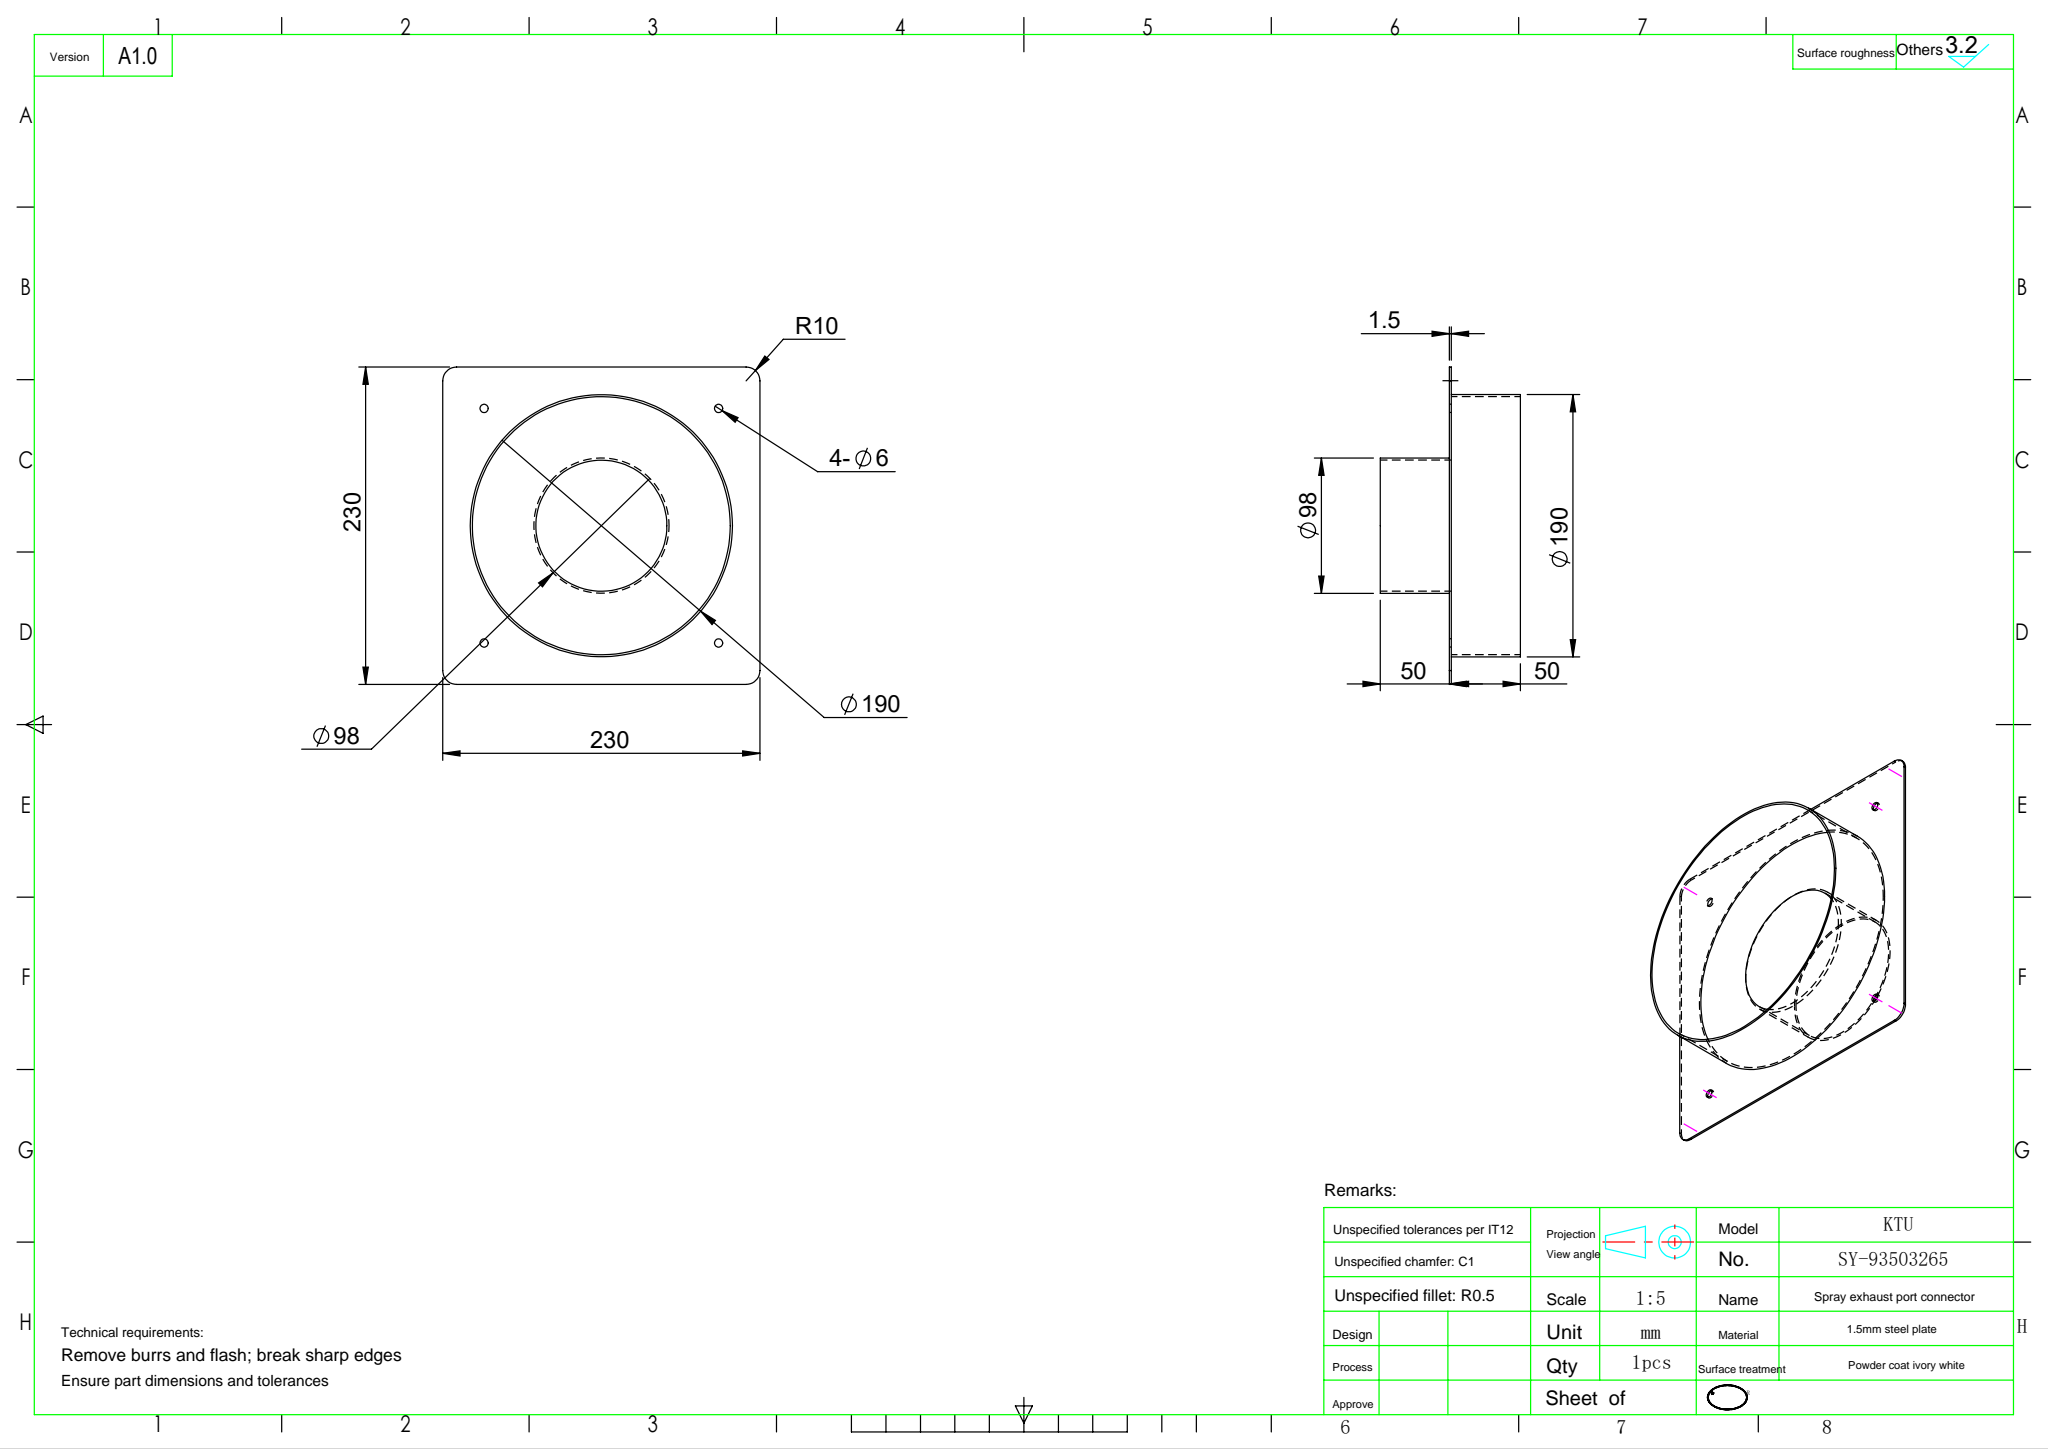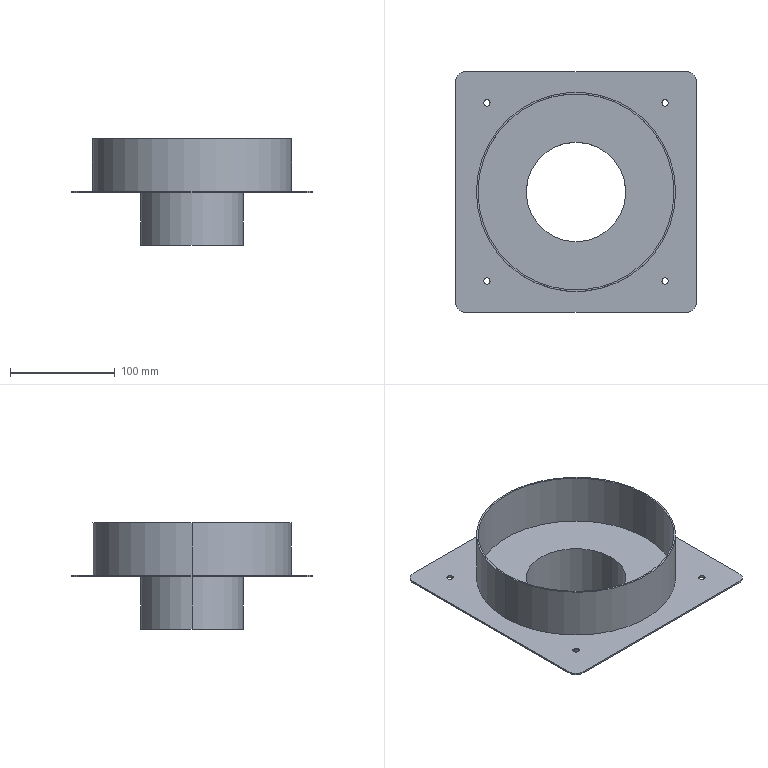Part | SolidWorks | features BossThin 2, FlatPattern 1, ICE 1, SMBaseFlange 1, SheetMetal 1 | 1 solid | 29 faces | box 230 x 230 x 101.5 mm | volume 135571 mm3 | cylinder 20 | plane 9 | commonest cylinder face diameters 6 x8 20 x4 95 x2 98 x2 187 x2 190 x2
STEP:
#1=CARTESIAN_POINT('',(-93.5,0.,50.));
#2=VERTEX_POINT('',#1);
#3=CARTESIAN_POINT('',(93.5,0.,50.));
#4=VERTEX_POINT('',#3);
#5=CARTESIAN_POINT('',(0.,0.,50.));
#6=DIRECTION('',(0.,0.,1.));
#7=DIRECTION('',(1.,0.,0.));
#8=AXIS2_PLACEMENT_3D('',#5,#6,#7);
#9=CIRCLE('',#8,93.5);
#10=EDGE_CURVE('',#2,#4,#9,.T.);
#11=ORIENTED_EDGE('',*,*,#10,.T.);
#12=CARTESIAN_POINT('',(93.5,0.,0.));
#13=VERTEX_POINT('',#12);
#14=CARTESIAN_POINT('',(93.5,0.,50.));
#15=DIRECTION('',(0.,0.,-1.));
#16=VECTOR('',#15,1000.);
#17=LINE('',#14,#16);
#18=EDGE_CURVE('',#4,#13,#17,.T.);
#19=ORIENTED_EDGE('',*,*,#18,.T.);
#20=CARTESIAN_POINT('',(-93.5,0.,0.));
#21=VERTEX_POINT('',#20);
#22=CARTESIAN_POINT('',(0.,0.,0.));
#23=DIRECTION('',(0.,0.,-1.));
#24=DIRECTION('',(1.,0.,0.));
#25=AXIS2_PLACEMENT_3D('',#22,#23,#24);
#26=CIRCLE('',#25,93.5);
#27=EDGE_CURVE('',#13,#21,#26,.T.);
#28=ORIENTED_EDGE('',*,*,#27,.T.);
#29=CARTESIAN_POINT('',(-93.5,0.,50.));
#30=DIRECTION('',(0.,0.,-1.));
#31=VECTOR('',#30,1000.);
#32=LINE('',#29,#31);
#33=EDGE_CURVE('',#2,#21,#32,.T.);
#34=ORIENTED_EDGE('',*,*,#33,.F.);
#35=EDGE_LOOP('',(#11,#19,#28,#34));
#36=FACE_OUTER_BOUND('',#35,.T.);
#37=CARTESIAN_POINT('',(0.,0.,50.));
#38=DIRECTION('',(0.,0.,-1.));
#39=DIRECTION('',(-1.,0.,0.));
#40=AXIS2_PLACEMENT_3D('',#37,#38,#39);
#41=CYLINDRICAL_SURFACE('',#40,93.5);
#42=ADVANCED_FACE('',(#36),#41,.F.);
#43=CARTESIAN_POINT('',(95.,0.,50.));
#44=VERTEX_POINT('',#43);
#45=CARTESIAN_POINT('',(-95.,0.,50.));
#46=VERTEX_POINT('',#45);
#47=CARTESIAN_POINT('',(0.,0.,50.));
#48=DIRECTION('',(0.,0.,1.));
#49=DIRECTION('',(1.,0.,0.));
#50=AXIS2_PLACEMENT_3D('',#47,#48,#49);
#51=CIRCLE('',#50,95.);
#52=EDGE_CURVE('',#44,#46,#51,.T.);
#53=ORIENTED_EDGE('',*,*,#52,.F.);
#54=CARTESIAN_POINT('',(95.,0.,0.));
#55=VERTEX_POINT('',#54);
#56=CARTESIAN_POINT('',(95.,0.,50.));
#57=DIRECTION('',(0.,0.,-1.));
#58=VECTOR('',#57,1000.);
#59=LINE('',#56,#58);
#60=EDGE_CURVE('',#44,#55,#59,.T.);
#61=ORIENTED_EDGE('',*,*,#60,.T.);
#62=CARTESIAN_POINT('',(-95.,0.,0.));
#63=VERTEX_POINT('',#62);
#64=CARTESIAN_POINT('',(0.,0.,0.));
#65=DIRECTION('',(0.,0.,1.));
#66=DIRECTION('',(1.,0.,0.));
#67=AXIS2_PLACEMENT_3D('',#64,#65,#66);
#68=CIRCLE('',#67,95.);
#69=EDGE_CURVE('',#55,#63,#68,.T.);
#70=ORIENTED_EDGE('',*,*,#69,.T.);
#71=CARTESIAN_POINT('',(-95.,0.,50.));
#72=DIRECTION('',(0.,0.,-1.));
#73=VECTOR('',#72,1000.);
#74=LINE('',#71,#73);
#75=EDGE_CURVE('',#46,#63,#74,.T.);
#76=ORIENTED_EDGE('',*,*,#75,.F.);
#77=EDGE_LOOP('',(#53,#61,#70,#76));
#78=FACE_OUTER_BOUND('',#77,.T.);
#79=CARTESIAN_POINT('',(0.,0.,50.));
#80=DIRECTION('',(0.,0.,-1.));
#81=DIRECTION('',(-1.,0.,0.));
#82=AXIS2_PLACEMENT_3D('',#79,#80,#81);
#83=CYLINDRICAL_SURFACE('',#82,95.);
#84=ADVANCED_FACE('',(#78),#83,.T.);
#85=CARTESIAN_POINT('',(-49.,0.,-51.5));
#86=VERTEX_POINT('',#85);
#87=CARTESIAN_POINT('',(49.,0.,-51.5));
#88=VERTEX_POINT('',#87);
#89=CARTESIAN_POINT('',(0.,0.,-51.5));
#90=DIRECTION('',(0.,0.,-1.));
#91=DIRECTION('',(-1.,0.,0.));
#92=AXIS2_PLACEMENT_3D('',#89,#90,#91);
#93=CIRCLE('',#92,49.);
#94=EDGE_CURVE('',#86,#88,#93,.T.);
#95=ORIENTED_EDGE('',*,*,#94,.F.);
#96=CARTESIAN_POINT('',(-49.,0.,-1.5));
#97=VERTEX_POINT('',#96);
#98=CARTESIAN_POINT('',(-49.,0.,-51.5));
#99=DIRECTION('',(0.,0.,1.));
#100=VECTOR('',#99,1000.);
#101=LINE('',#98,#100);
#102=EDGE_CURVE('',#86,#97,#101,.T.);
#103=ORIENTED_EDGE('',*,*,#102,.T.);
#104=CARTESIAN_POINT('',(49.,0.,-1.5));
#105=VERTEX_POINT('',#104);
#106=CARTESIAN_POINT('',(0.,0.,-1.5));
#107=DIRECTION('',(0.,0.,-1.));
#108=DIRECTION('',(1.,0.,0.));
#109=AXIS2_PLACEMENT_3D('',#106,#107,#108);
#110=CIRCLE('',#109,49.);
#111=EDGE_CURVE('',#97,#105,#110,.T.);
#112=ORIENTED_EDGE('',*,*,#111,.T.);
#113=CARTESIAN_POINT('',(49.,0.,-51.5));
#114=DIRECTION('',(0.,0.,1.));
#115=VECTOR('',#114,1000.);
#116=LINE('',#113,#115);
#117=EDGE_CURVE('',#88,#105,#116,.T.);
#118=ORIENTED_EDGE('',*,*,#117,.F.);
#119=EDGE_LOOP('',(#95,#103,#112,#118));
#120=FACE_OUTER_BOUND('',#119,.T.);
#121=CARTESIAN_POINT('',(0.,0.,-51.5));
#122=DIRECTION('',(0.,0.,1.));
#123=DIRECTION('',(1.,0.,0.));
#124=AXIS2_PLACEMENT_3D('',#121,#122,#123);
#125=CYLINDRICAL_SURFACE('',#124,49.);
#126=ADVANCED_FACE('',(#120),#125,.T.);
#127=CARTESIAN_POINT('',(82.,85.,0.));
#128=VERTEX_POINT('',#127);
#129=CARTESIAN_POINT('',(88.,85.,0.));
#130=VERTEX_POINT('',#129);
#131=CARTESIAN_POINT('',(85.,85.,0.));
#132=DIRECTION('',(0.,0.,1.));
#133=DIRECTION('',(1.,0.,0.));
#134=AXIS2_PLACEMENT_3D('',#131,#132,#133);
#135=CIRCLE('',#134,3.);
#136=EDGE_CURVE('',#128,#130,#135,.T.);
#137=ORIENTED_EDGE('',*,*,#136,.T.);
#138=CARTESIAN_POINT('',(88.,85.,-1.5));
#139=VERTEX_POINT('',#138);
#140=CARTESIAN_POINT('',(88.,85.,46.5));
#141=DIRECTION('',(0.,0.,-1.));
#142=VECTOR('',#141,1000.);
#143=LINE('',#140,#142);
#144=EDGE_CURVE('',#130,#139,#143,.T.);
#145=ORIENTED_EDGE('',*,*,#144,.T.);
#146=CARTESIAN_POINT('',(82.,85.,-1.5));
#147=VERTEX_POINT('',#146);
#148=CARTESIAN_POINT('',(85.,85.,-1.5));
#149=DIRECTION('',(0.,0.,-1.));
#150=DIRECTION('',(-1.,0.,0.));
#151=AXIS2_PLACEMENT_3D('',#148,#149,#150);
#152=CIRCLE('',#151,3.);
#153=EDGE_CURVE('',#139,#147,#152,.T.);
#154=ORIENTED_EDGE('',*,*,#153,.T.);
#155=CARTESIAN_POINT('',(82.,85.,46.5));
#156=DIRECTION('',(0.,0.,-1.));
#157=VECTOR('',#156,1000.);
#158=LINE('',#155,#157);
#159=EDGE_CURVE('',#128,#147,#158,.T.);
#160=ORIENTED_EDGE('',*,*,#159,.F.);
#161=EDGE_LOOP('',(#137,#145,#154,#160));
#162=FACE_OUTER_BOUND('',#161,.T.);
#163=CARTESIAN_POINT('',(85.,85.,46.5));
#164=DIRECTION('',(0.,0.,-1.));
#165=DIRECTION('',(-1.,0.,0.));
#166=AXIS2_PLACEMENT_3D('',#163,#164,#165);
#167=CYLINDRICAL_SURFACE('',#166,3.);
#168=ADVANCED_FACE('',(#162),#167,.F.);
#169=CARTESIAN_POINT('',(82.,-85.,0.));
#170=VERTEX_POINT('',#169);
#171=CARTESIAN_POINT('',(88.,-85.,0.));
#172=VERTEX_POINT('',#171);
#173=CARTESIAN_POINT('',(85.,-85.,0.));
#174=DIRECTION('',(0.,0.,1.));
#175=DIRECTION('',(1.,0.,0.));
#176=AXIS2_PLACEMENT_3D('',#173,#174,#175);
#177=CIRCLE('',#176,3.);
#178=EDGE_CURVE('',#170,#172,#177,.T.);
#179=ORIENTED_EDGE('',*,*,#178,.T.);
#180=CARTESIAN_POINT('',(88.,-85.,-1.5));
#181=VERTEX_POINT('',#180);
#182=CARTESIAN_POINT('',(88.,-85.,46.5));
#183=DIRECTION('',(0.,0.,-1.));
#184=VECTOR('',#183,1000.);
#185=LINE('',#182,#184);
#186=EDGE_CURVE('',#172,#181,#185,.T.);
#187=ORIENTED_EDGE('',*,*,#186,.T.);
#188=CARTESIAN_POINT('',(82.,-85.,-1.5));
#189=VERTEX_POINT('',#188);
#190=CARTESIAN_POINT('',(85.,-85.,-1.5));
#191=DIRECTION('',(0.,0.,-1.));
#192=DIRECTION('',(-1.,0.,0.));
#193=AXIS2_PLACEMENT_3D('',#190,#191,#192);
#194=CIRCLE('',#193,3.);
#195=EDGE_CURVE('',#181,#189,#194,.T.);
#196=ORIENTED_EDGE('',*,*,#195,.T.);
#197=CARTESIAN_POINT('',(82.,-85.,46.5));
#198=DIRECTION('',(0.,0.,-1.));
#199=VECTOR('',#198,1000.);
#200=LINE('',#197,#199);
#201=EDGE_CURVE('',#170,#189,#200,.T.);
#202=ORIENTED_EDGE('',*,*,#201,.F.);
#203=EDGE_LOOP('',(#179,#187,#196,#202));
#204=FACE_OUTER_BOUND('',#203,.T.);
#205=CARTESIAN_POINT('',(85.,-85.,46.5));
#206=DIRECTION('',(0.,0.,-1.));
#207=DIRECTION('',(-1.,0.,0.));
#208=AXIS2_PLACEMENT_3D('',#205,#206,#207);
#209=CYLINDRICAL_SURFACE('',#208,3.);
#210=ADVANCED_FACE('',(#204),#209,.F.);
#211=CARTESIAN_POINT('',(-88.,-85.,0.));
#212=VERTEX_POINT('',#211);
#213=CARTESIAN_POINT('',(-82.,-85.,0.));
#214=VERTEX_POINT('',#213);
#215=CARTESIAN_POINT('',(-85.,-85.,0.));
#216=DIRECTION('',(0.,0.,1.));
#217=DIRECTION('',(1.,0.,0.));
#218=AXIS2_PLACEMENT_3D('',#215,#216,#217);
#219=CIRCLE('',#218,3.);
#220=EDGE_CURVE('',#212,#214,#219,.T.);
#221=ORIENTED_EDGE('',*,*,#220,.T.);
#222=CARTESIAN_POINT('',(-82.,-85.,-1.5));
#223=VERTEX_POINT('',#222);
#224=CARTESIAN_POINT('',(-82.,-85.,46.5));
#225=DIRECTION('',(0.,0.,-1.));
#226=VECTOR('',#225,1000.);
#227=LINE('',#224,#226);
#228=EDGE_CURVE('',#214,#223,#227,.T.);
#229=ORIENTED_EDGE('',*,*,#228,.T.);
#230=CARTESIAN_POINT('',(-88.,-85.,-1.5));
#231=VERTEX_POINT('',#230);
#232=CARTESIAN_POINT('',(-85.,-85.,-1.5));
#233=DIRECTION('',(0.,0.,-1.));
#234=DIRECTION('',(-1.,0.,0.));
#235=AXIS2_PLACEMENT_3D('',#232,#233,#234);
#236=CIRCLE('',#235,3.);
#237=EDGE_CURVE('',#223,#231,#236,.T.);
#238=ORIENTED_EDGE('',*,*,#237,.T.);
#239=CARTESIAN_POINT('',(-88.,-85.,46.5));
#240=DIRECTION('',(0.,0.,-1.));
#241=VECTOR('',#240,1000.);
#242=LINE('',#239,#241);
#243=EDGE_CURVE('',#212,#231,#242,.T.);
#244=ORIENTED_EDGE('',*,*,#243,.F.);
#245=EDGE_LOOP('',(#221,#229,#238,#244));
#246=FACE_OUTER_BOUND('',#245,.T.);
#247=CARTESIAN_POINT('',(-85.,-85.,46.5));
#248=DIRECTION('',(0.,0.,-1.));
#249=DIRECTION('',(-1.,0.,0.));
#250=AXIS2_PLACEMENT_3D('',#247,#248,#249);
#251=CYLINDRICAL_SURFACE('',#250,3.);
#252=ADVANCED_FACE('',(#246),#251,.F.);
#253=CARTESIAN_POINT('',(-88.,85.,0.));
#254=VERTEX_POINT('',#253);
#255=CARTESIAN_POINT('',(-82.,85.,0.));
#256=VERTEX_POINT('',#255);
#257=CARTESIAN_POINT('',(-85.,85.,0.));
#258=DIRECTION('',(0.,0.,1.));
#259=DIRECTION('',(1.,0.,0.));
#260=AXIS2_PLACEMENT_3D('',#257,#258,#259);
#261=CIRCLE('',#260,3.);
#262=EDGE_CURVE('',#254,#256,#261,.T.);
#263=ORIENTED_EDGE('',*,*,#262,.T.);
#264=CARTESIAN_POINT('',(-82.,85.,-1.5));
#265=VERTEX_POINT('',#264);
#266=CARTESIAN_POINT('',(-82.,85.,46.5));
#267=DIRECTION('',(0.,0.,-1.));
#268=VECTOR('',#267,1000.);
#269=LINE('',#266,#268);
#270=EDGE_CURVE('',#256,#265,#269,.T.);
#271=ORIENTED_EDGE('',*,*,#270,.T.);
#272=CARTESIAN_POINT('',(-88.,85.,-1.5));
#273=VERTEX_POINT('',#272);
#274=CARTESIAN_POINT('',(-85.,85.,-1.5));
#275=DIRECTION('',(0.,0.,-1.));
#276=DIRECTION('',(-1.,0.,0.));
#277=AXIS2_PLACEMENT_3D('',#274,#275,#276);
#278=CIRCLE('',#277,3.);
#279=EDGE_CURVE('',#265,#273,#278,.T.);
#280=ORIENTED_EDGE('',*,*,#279,.T.);
#281=CARTESIAN_POINT('',(-88.,85.,46.5));
#282=DIRECTION('',(0.,0.,-1.));
#283=VECTOR('',#282,1000.);
#284=LINE('',#281,#283);
#285=EDGE_CURVE('',#254,#273,#284,.T.);
#286=ORIENTED_EDGE('',*,*,#285,.F.);
#287=EDGE_LOOP('',(#263,#271,#280,#286));
#288=FACE_OUTER_BOUND('',#287,.T.);
#289=CARTESIAN_POINT('',(-85.,85.,46.5));
#290=DIRECTION('',(0.,0.,-1.));
#291=DIRECTION('',(-1.,0.,0.));
#292=AXIS2_PLACEMENT_3D('',#289,#290,#291);
#293=CYLINDRICAL_SURFACE('',#292,3.);
#294=ADVANCED_FACE('',(#288),#293,.F.);
#295=CARTESIAN_POINT('',(47.5,0.,-51.5));
#296=VERTEX_POINT('',#295);
#297=CARTESIAN_POINT('',(-47.5,0.,-51.5));
#298=VERTEX_POINT('',#297);
#299=CARTESIAN_POINT('',(0.,0.,-51.5));
#300=DIRECTION('',(0.,0.,-1.));
#301=DIRECTION('',(-1.,0.,0.));
#302=AXIS2_PLACEMENT_3D('',#299,#300,#301);
#303=CIRCLE('',#302,47.5);
#304=EDGE_CURVE('',#296,#298,#303,.T.);
#305=ORIENTED_EDGE('',*,*,#304,.T.);
#306=CARTESIAN_POINT('',(-47.5,0.,0.));
#307=VERTEX_POINT('',#306);
#308=CARTESIAN_POINT('',(-47.5,0.,-1.5));
#309=DIRECTION('',(0.,0.,1.));
#310=VECTOR('',#309,1000.);
#311=LINE('',#308,#310);
#312=EDGE_CURVE('',#298,#307,#311,.T.);
#313=ORIENTED_EDGE('',*,*,#312,.T.);
#314=CARTESIAN_POINT('',(47.5,0.,0.));
#315=VERTEX_POINT('',#314);
#316=CARTESIAN_POINT('',(0.,0.,0.));
#317=DIRECTION('',(0.,0.,1.));
#318=DIRECTION('',(1.,0.,0.));
#319=AXIS2_PLACEMENT_3D('',#316,#317,#318);
#320=CIRCLE('',#319,47.5);
#321=EDGE_CURVE('',#307,#315,#320,.T.);
#322=ORIENTED_EDGE('',*,*,#321,.T.);
#323=CARTESIAN_POINT('',(47.5,0.,-1.5));
#324=DIRECTION('',(0.,0.,1.));
#325=VECTOR('',#324,1000.);
#326=LINE('',#323,#325);
#327=EDGE_CURVE('',#296,#315,#326,.T.);
#328=ORIENTED_EDGE('',*,*,#327,.F.);
#329=EDGE_LOOP('',(#305,#313,#322,#328));
#330=FACE_OUTER_BOUND('',#329,.T.);
#331=CARTESIAN_POINT('',(0.,0.,-1.5));
#332=DIRECTION('',(0.,0.,1.));
#333=DIRECTION('',(1.,0.,0.));
#334=AXIS2_PLACEMENT_3D('',#331,#332,#333);
#335=CYLINDRICAL_SURFACE('',#334,47.5);
#336=ADVANCED_FACE('',(#330),#335,.F.);
#337=CARTESIAN_POINT('',(0.,0.,0.));
#338=DIRECTION('',(0.,0.,1.));
#339=DIRECTION('',(1.,0.,0.));
#340=AXIS2_PLACEMENT_3D('',#337,#338,#339);
#341=CIRCLE('',#340,47.5);
#342=EDGE_CURVE('',#315,#307,#341,.T.);
#343=ORIENTED_EDGE('',*,*,#342,.F.);
#344=ORIENTED_EDGE('',*,*,#321,.F.);
#345=EDGE_LOOP('',(#343,#344));
#346=FACE_BOUND('',#345,.T.);
#347=CARTESIAN_POINT('',(0.,0.,0.));
#348=DIRECTION('',(0.,0.,-1.));
#349=DIRECTION('',(1.,0.,0.));
#350=AXIS2_PLACEMENT_3D('',#347,#348,#349);
#351=CIRCLE('',#350,93.5);
#352=EDGE_CURVE('',#21,#13,#351,.T.);
#353=ORIENTED_EDGE('',*,*,#352,.F.);
#354=ORIENTED_EDGE('',*,*,#27,.F.);
#355=EDGE_LOOP('',(#353,#354));
#356=FACE_OUTER_BOUND('',#355,.T.);
#357=CARTESIAN_POINT('',(-105.,-105.,0.));
#358=DIRECTION('',(0.,0.,1.));
#359=DIRECTION('',(1.,0.,0.));
#360=AXIS2_PLACEMENT_3D('',#357,#358,#359);
#361=PLANE('',#360);
#362=ADVANCED_FACE('',(#346,#356),#361,.T.);
#363=CARTESIAN_POINT('',(-115.,-105.,-1.5));
#364=VERTEX_POINT('',#363);
#365=CARTESIAN_POINT('',(-105.,-115.,-1.5));
#366=VERTEX_POINT('',#365);
#367=CARTESIAN_POINT('',(-105.,-105.,-1.5));
#368=DIRECTION('',(0.,0.,1.));
#369=DIRECTION('',(1.,0.,0.));
#370=AXIS2_PLACEMENT_3D('',#367,#368,#369);
#371=CIRCLE('',#370,10.);
#372=EDGE_CURVE('',#364,#366,#371,.T.);
#373=ORIENTED_EDGE('',*,*,#372,.F.);
#374=CARTESIAN_POINT('',(-115.,105.,-1.5));
#375=VERTEX_POINT('',#374);
#376=CARTESIAN_POINT('',(-115.,-105.,-1.5));
#377=DIRECTION('',(0.,-1.,0.));
#378=VECTOR('',#377,1000.);
#379=LINE('',#376,#378);
#380=EDGE_CURVE('',#375,#364,#379,.T.);
#381=ORIENTED_EDGE('',*,*,#380,.F.);
#382=CARTESIAN_POINT('',(-105.,115.,-1.5));
#383=VERTEX_POINT('',#382);
#384=CARTESIAN_POINT('',(-105.,105.,-1.5));
#385=DIRECTION('',(0.,0.,1.));
#386=DIRECTION('',(-1.,0.,0.));
#387=AXIS2_PLACEMENT_3D('',#384,#385,#386);
#388=CIRCLE('',#387,10.);
#389=EDGE_CURVE('',#383,#375,#388,.T.);
#390=ORIENTED_EDGE('',*,*,#389,.F.);
#391=CARTESIAN_POINT('',(105.,115.,-1.5));
#392=VERTEX_POINT('',#391);
#393=CARTESIAN_POINT('',(-105.,115.,-1.5));
#394=DIRECTION('',(-1.,0.,0.));
#395=VECTOR('',#394,1000.);
#396=LINE('',#393,#395);
#397=EDGE_CURVE('',#392,#383,#396,.T.);
#398=ORIENTED_EDGE('',*,*,#397,.F.);
#399=CARTESIAN_POINT('',(115.,105.,-1.5));
#400=VERTEX_POINT('',#399);
#401=CARTESIAN_POINT('',(105.,105.,-1.5));
#402=DIRECTION('',(0.,0.,1.));
#403=DIRECTION('',(1.,0.,0.));
#404=AXIS2_PLACEMENT_3D('',#401,#402,#403);
#405=CIRCLE('',#404,10.);
#406=EDGE_CURVE('',#400,#392,#405,.T.);
#407=ORIENTED_EDGE('',*,*,#406,.F.);
#408=CARTESIAN_POINT('',(115.,-105.,-1.5));
#409=VERTEX_POINT('',#408);
#410=CARTESIAN_POINT('',(115.,-105.,-1.5));
#411=DIRECTION('',(0.,1.,0.));
#412=VECTOR('',#411,1000.);
#413=LINE('',#410,#412);
#414=EDGE_CURVE('',#409,#400,#413,.T.);
#415=ORIENTED_EDGE('',*,*,#414,.F.);
#416=CARTESIAN_POINT('',(105.,-115.,-1.5));
#417=VERTEX_POINT('',#416);
#418=CARTESIAN_POINT('',(105.,-105.,-1.5));
#419=DIRECTION('',(0.,0.,1.));
#420=DIRECTION('',(1.,0.,0.));
#421=AXIS2_PLACEMENT_3D('',#418,#419,#420);
#422=CIRCLE('',#421,10.);
#423=EDGE_CURVE('',#417,#409,#422,.T.);
#424=ORIENTED_EDGE('',*,*,#423,.F.);
#425=CARTESIAN_POINT('',(-105.,-115.,-1.5));
#426=DIRECTION('',(1.,0.,0.));
#427=VECTOR('',#426,1000.);
#428=LINE('',#425,#427);
#429=EDGE_CURVE('',#366,#417,#428,.T.);
#430=ORIENTED_EDGE('',*,*,#429,.F.);
#431=EDGE_LOOP('',(#373,#381,#390,#398,#407,#415,#424,#430));
#432=FACE_OUTER_BOUND('',#431,.T.);
#433=CARTESIAN_POINT('',(-85.,85.,-1.5));
#434=DIRECTION('',(0.,0.,-1.));
#435=DIRECTION('',(-1.,0.,0.));
#436=AXIS2_PLACEMENT_3D('',#433,#434,#435);
#437=CIRCLE('',#436,3.);
#438=EDGE_CURVE('',#273,#265,#437,.T.);
#439=ORIENTED_EDGE('',*,*,#438,.F.);
#440=ORIENTED_EDGE('',*,*,#279,.F.);
#441=EDGE_LOOP('',(#439,#440));
#442=FACE_BOUND('',#441,.T.);
#443=CARTESIAN_POINT('',(-85.,-85.,-1.5));
#444=DIRECTION('',(0.,0.,-1.));
#445=DIRECTION('',(-1.,0.,0.));
#446=AXIS2_PLACEMENT_3D('',#443,#444,#445);
#447=CIRCLE('',#446,3.);
#448=EDGE_CURVE('',#231,#223,#447,.T.);
#449=ORIENTED_EDGE('',*,*,#448,.F.);
#450=ORIENTED_EDGE('',*,*,#237,.F.);
#451=EDGE_LOOP('',(#449,#450));
#452=FACE_BOUND('',#451,.T.);
#453=CARTESIAN_POINT('',(85.,-85.,-1.5));
#454=DIRECTION('',(0.,0.,-1.));
#455=DIRECTION('',(-1.,0.,0.));
#456=AXIS2_PLACEMENT_3D('',#453,#454,#455);
#457=CIRCLE('',#456,3.);
#458=EDGE_CURVE('',#189,#181,#457,.T.);
#459=ORIENTED_EDGE('',*,*,#458,.F.);
#460=ORIENTED_EDGE('',*,*,#195,.F.);
#461=EDGE_LOOP('',(#459,#460));
#462=FACE_BOUND('',#461,.T.);
#463=CARTESIAN_POINT('',(85.,85.,-1.5));
#464=DIRECTION('',(0.,0.,-1.));
#465=DIRECTION('',(-1.,0.,0.));
#466=AXIS2_PLACEMENT_3D('',#463,#464,#465);
#467=CIRCLE('',#466,3.);
#468=EDGE_CURVE('',#147,#139,#467,.T.);
#469=ORIENTED_EDGE('',*,*,#468,.F.);
#470=ORIENTED_EDGE('',*,*,#153,.F.);
#471=EDGE_LOOP('',(#469,#470));
#472=FACE_BOUND('',#471,.T.);
#473=CARTESIAN_POINT('',(0.,0.,-1.5));
#474=DIRECTION('',(0.,0.,-1.));
#475=DIRECTION('',(1.,0.,0.));
#476=AXIS2_PLACEMENT_3D('',#473,#474,#475);
#477=CIRCLE('',#476,49.);
#478=EDGE_CURVE('',#105,#97,#477,.T.);
#479=ORIENTED_EDGE('',*,*,#478,.F.);
#480=ORIENTED_EDGE('',*,*,#111,.F.);
#481=EDGE_LOOP('',(#479,#480));
#482=FACE_BOUND('',#481,.T.);
#483=CARTESIAN_POINT('',(-105.,-105.,-1.5));
#484=DIRECTION('',(0.,0.,1.));
#485=DIRECTION('',(1.,0.,0.));
#486=AXIS2_PLACEMENT_3D('',#483,#484,#485);
#487=PLANE('',#486);
#488=ADVANCED_FACE('',(#432,#442,#452,#462,#472,#482),#487,.F.);
#489=CARTESIAN_POINT('',(-115.,-105.,0.));
#490=VERTEX_POINT('',#489);
#491=CARTESIAN_POINT('',(-105.,-115.,0.));
#492=VERTEX_POINT('',#491);
#493=CARTESIAN_POINT('',(-105.,-105.,0.));
#494=DIRECTION('',(0.,0.,1.));
#495=DIRECTION('',(1.,0.,0.));
#496=AXIS2_PLACEMENT_3D('',#493,#494,#495);
#497=CIRCLE('',#496,10.);
#498=EDGE_CURVE('',#490,#492,#497,.T.);
#499=ORIENTED_EDGE('',*,*,#498,.F.);
#500=CARTESIAN_POINT('',(-115.,-105.,-1.5));
#501=DIRECTION('',(0.,0.,1.));
#502=VECTOR('',#501,1000.);
#503=LINE('',#500,#502);
#504=EDGE_CURVE('',#364,#490,#503,.T.);
#505=ORIENTED_EDGE('',*,*,#504,.F.);
#506=ORIENTED_EDGE('',*,*,#372,.T.);
#507=CARTESIAN_POINT('',(-105.,-115.,-1.5));
#508=DIRECTION('',(0.,0.,1.));
#509=VECTOR('',#508,1000.);
#510=LINE('',#507,#509);
#511=EDGE_CURVE('',#366,#492,#510,.T.);
#512=ORIENTED_EDGE('',*,*,#511,.T.);
#513=EDGE_LOOP('',(#499,#505,#506,#512));
#514=FACE_OUTER_BOUND('',#513,.T.);
#515=CARTESIAN_POINT('',(-105.,-105.,-1.5));
#516=DIRECTION('',(0.,0.,1.));
#517=DIRECTION('',(1.,0.,0.));
#518=AXIS2_PLACEMENT_3D('',#515,#516,#517);
#519=CYLINDRICAL_SURFACE('',#518,10.);
#520=ADVANCED_FACE('',(#514),#519,.T.);
#521=CARTESIAN_POINT('',(-115.,105.,0.));
#522=VERTEX_POINT('',#521);
#523=CARTESIAN_POINT('',(-115.,-105.,0.));
#524=DIRECTION('',(0.,-1.,0.));
#525=VECTOR('',#524,1000.);
#526=LINE('',#523,#525);
#527=EDGE_CURVE('',#522,#490,#526,.T.);
#528=ORIENTED_EDGE('',*,*,#527,.F.);
#529=CARTESIAN_POINT('',(-115.,105.,-1.5));
#530=DIRECTION('',(0.,0.,1.));
#531=VECTOR('',#530,1000.);
#532=LINE('',#529,#531);
#533=EDGE_CURVE('',#375,#522,#532,.T.);
#534=ORIENTED_EDGE('',*,*,#533,.F.);
#535=ORIENTED_EDGE('',*,*,#380,.T.);
#536=ORIENTED_EDGE('',*,*,#504,.T.);
#537=EDGE_LOOP('',(#528,#534,#535,#536));
#538=FACE_OUTER_BOUND('',#537,.T.);
#539=CARTESIAN_POINT('',(-115.,-105.,-1.5));
#540=DIRECTION('',(-1.,0.,0.));
#541=DIRECTION('',(0.,0.,1.));
#542=AXIS2_PLACEMENT_3D('',#539,#540,#541);
#543=PLANE('',#542);
#544=ADVANCED_FACE('',(#538),#543,.T.);
#545=CARTESIAN_POINT('',(-105.,115.,0.));
#546=VERTEX_POINT('',#545);
#547=CARTESIAN_POINT('',(-105.,105.,0.));
#548=DIRECTION('',(0.,0.,1.));
#549=DIRECTION('',(-1.,0.,0.));
#550=AXIS2_PLACEMENT_3D('',#547,#548,#549);
#551=CIRCLE('',#550,10.);
#552=EDGE_CURVE('',#546,#522,#551,.T.);
#553=ORIENTED_EDGE('',*,*,#552,.F.);
#554=CARTESIAN_POINT('',(-105.,115.,-1.5));
#555=DIRECTION('',(0.,0.,1.));
#556=VECTOR('',#555,1000.);
#557=LINE('',#554,#556);
#558=EDGE_CURVE('',#383,#546,#557,.T.);
#559=ORIENTED_EDGE('',*,*,#558,.F.);
#560=ORIENTED_EDGE('',*,*,#389,.T.);
#561=ORIENTED_EDGE('',*,*,#533,.T.);
#562=EDGE_LOOP('',(#553,#559,#560,#561));
#563=FACE_OUTER_BOUND('',#562,.T.);
#564=CARTESIAN_POINT('',(-105.,105.,-1.5));
#565=DIRECTION('',(0.,0.,1.));
#566=DIRECTION('',(1.,0.,0.));
#567=AXIS2_PLACEMENT_3D('',#564,#565,#566);
#568=CYLINDRICAL_SURFACE('',#567,10.);
#569=ADVANCED_FACE('',(#563),#568,.T.);
#570=CARTESIAN_POINT('',(105.,115.,0.));
#571=VERTEX_POINT('',#570);
#572=CARTESIAN_POINT('',(-105.,115.,0.));
#573=DIRECTION('',(-1.,0.,0.));
#574=VECTOR('',#573,1000.);
#575=LINE('',#572,#574);
#576=EDGE_CURVE('',#571,#546,#575,.T.);
#577=ORIENTED_EDGE('',*,*,#576,.F.);
#578=CARTESIAN_POINT('',(105.,115.,-1.5));
#579=DIRECTION('',(0.,0.,1.));
#580=VECTOR('',#579,1000.);
#581=LINE('',#578,#580);
#582=EDGE_CURVE('',#392,#571,#581,.T.);
#583=ORIENTED_EDGE('',*,*,#582,.F.);
#584=ORIENTED_EDGE('',*,*,#397,.T.);
#585=ORIENTED_EDGE('',*,*,#558,.T.);
#586=EDGE_LOOP('',(#577,#583,#584,#585));
#587=FACE_OUTER_BOUND('',#586,.T.);
#588=CARTESIAN_POINT('',(-105.,115.,-1.5));
#589=DIRECTION('',(0.,1.,0.));
#590=DIRECTION('',(0.,0.,1.));
#591=AXIS2_PLACEMENT_3D('',#588,#589,#590);
#592=PLANE('',#591);
#593=ADVANCED_FACE('',(#587),#592,.T.);
#594=CARTESIAN_POINT('',(115.,105.,0.));
#595=VERTEX_POINT('',#594);
#596=CARTESIAN_POINT('',(105.,105.,0.));
#597=DIRECTION('',(0.,0.,1.));
#598=DIRECTION('',(1.,0.,0.));
#599=AXIS2_PLACEMENT_3D('',#596,#597,#598);
#600=CIRCLE('',#599,10.);
#601=EDGE_CURVE('',#595,#571,#600,.T.);
#602=ORIENTED_EDGE('',*,*,#601,.F.);
#603=CARTESIAN_POINT('',(115.,105.,-1.5));
#604=DIRECTION('',(0.,0.,1.));
#605=VECTOR('',#604,1000.);
#606=LINE('',#603,#605);
#607=EDGE_CURVE('',#400,#595,#606,.T.);
#608=ORIENTED_EDGE('',*,*,#607,.F.);
#609=ORIENTED_EDGE('',*,*,#406,.T.);
#610=ORIENTED_EDGE('',*,*,#582,.T.);
#611=EDGE_LOOP('',(#602,#608,#609,#610));
#612=FACE_OUTER_BOUND('',#611,.T.);
#613=CARTESIAN_POINT('',(105.,105.,-1.5));
#614=DIRECTION('',(0.,0.,1.));
#615=DIRECTION('',(1.,0.,0.));
#616=AXIS2_PLACEMENT_3D('',#613,#614,#615);
#617=CYLINDRICAL_SURFACE('',#616,10.);
#618=ADVANCED_FACE('',(#612),#617,.T.);
#619=CARTESIAN_POINT('',(115.,-105.,0.));
#620=VERTEX_POINT('',#619);
#621=CARTESIAN_POINT('',(115.,-105.,0.));
#622=DIRECTION('',(0.,1.,0.));
#623=VECTOR('',#622,1000.);
#624=LINE('',#621,#623);
#625=EDGE_CURVE('',#620,#595,#624,.T.);
#626=ORIENTED_EDGE('',*,*,#625,.F.);
#627=CARTESIAN_POINT('',(115.,-105.,-1.5));
#628=DIRECTION('',(0.,0.,1.));
#629=VECTOR('',#628,1000.);
#630=LINE('',#627,#629);
#631=EDGE_CURVE('',#409,#620,#630,.T.);
#632=ORIENTED_EDGE('',*,*,#631,.F.);
#633=ORIENTED_EDGE('',*,*,#414,.T.);
#634=ORIENTED_EDGE('',*,*,#607,.T.);
#635=EDGE_LOOP('',(#626,#632,#633,#634));
#636=FACE_OUTER_BOUND('',#635,.T.);
#637=CARTESIAN_POINT('',(115.,-105.,-1.5));
#638=DIRECTION('',(1.,0.,0.));
#639=DIRECTION('',(0.,0.,-1.));
#640=AXIS2_PLACEMENT_3D('',#637,#638,#639);
#641=PLANE('',#640);
#642=ADVANCED_FACE('',(#636),#641,.T.);
#643=CARTESIAN_POINT('',(105.,-115.,0.));
#644=VERTEX_POINT('',#643);
#645=CARTESIAN_POINT('',(105.,-105.,0.));
#646=DIRECTION('',(0.,0.,1.));
#647=DIRECTION('',(1.,0.,0.));
#648=AXIS2_PLACEMENT_3D('',#645,#646,#647);
#649=CIRCLE('',#648,10.);
#650=EDGE_CURVE('',#644,#620,#649,.T.);
#651=ORIENTED_EDGE('',*,*,#650,.F.);
#652=CARTESIAN_POINT('',(105.,-115.,-1.5));
#653=DIRECTION('',(0.,0.,1.));
#654=VECTOR('',#653,1000.);
#655=LINE('',#652,#654);
#656=EDGE_CURVE('',#417,#644,#655,.T.);
#657=ORIENTED_EDGE('',*,*,#656,.F.);
#658=ORIENTED_EDGE('',*,*,#423,.T.);
#659=ORIENTED_EDGE('',*,*,#631,.T.);
#660=EDGE_LOOP('',(#651,#657,#658,#659));
#661=FACE_OUTER_BOUND('',#660,.T.);
#662=CARTESIAN_POINT('',(105.,-105.,-1.5));
#663=DIRECTION('',(0.,0.,1.));
#664=DIRECTION('',(1.,0.,0.));
#665=AXIS2_PLACEMENT_3D('',#662,#663,#664);
#666=CYLINDRICAL_SURFACE('',#665,10.);
#667=ADVANCED_FACE('',(#661),#666,.T.);
#668=CARTESIAN_POINT('',(-105.,-115.,0.));
#669=DIRECTION('',(1.,0.,0.));
#670=VECTOR('',#669,1000.);
#671=LINE('',#668,#670);
#672=EDGE_CURVE('',#492,#644,#671,.T.);
#673=ORIENTED_EDGE('',*,*,#672,.F.);
#674=ORIENTED_EDGE('',*,*,#511,.F.);
#675=ORIENTED_EDGE('',*,*,#429,.T.);
#676=ORIENTED_EDGE('',*,*,#656,.T.);
#677=EDGE_LOOP('',(#673,#674,#675,#676));
#678=FACE_OUTER_BOUND('',#677,.T.);
#679=CARTESIAN_POINT('',(-105.,-115.,-1.5));
#680=DIRECTION('',(0.,-1.,0.));
#681=DIRECTION('',(0.,0.,-1.));
#682=AXIS2_PLACEMENT_3D('',#679,#680,#681);
#683=PLANE('',#682);
#684=ADVANCED_FACE('',(#678),#683,.T.);
#685=CARTESIAN_POINT('',(0.,0.,0.));
#686=DIRECTION('',(0.,0.,1.));
#687=DIRECTION('',(1.,0.,0.));
#688=AXIS2_PLACEMENT_3D('',#685,#686,#687);
#689=CIRCLE('',#688,95.);
#690=EDGE_CURVE('',#63,#55,#689,.T.);
#691=ORIENTED_EDGE('',*,*,#690,.F.);
#692=ORIENTED_EDGE('',*,*,#69,.F.);
#693=EDGE_LOOP('',(#691,#692));
#694=FACE_BOUND('',#693,.T.);
#695=ORIENTED_EDGE('',*,*,#136,.F.);
#696=CARTESIAN_POINT('',(85.,85.,0.));
#697=DIRECTION('',(0.,0.,1.));
#698=DIRECTION('',(1.,0.,0.));
#699=AXIS2_PLACEMENT_3D('',#696,#697,#698);
#700=CIRCLE('',#699,3.);
#701=EDGE_CURVE('',#130,#128,#700,.T.);
#702=ORIENTED_EDGE('',*,*,#701,.F.);
#703=EDGE_LOOP('',(#695,#702));
#704=FACE_BOUND('',#703,.T.);
#705=ORIENTED_EDGE('',*,*,#178,.F.);
#706=CARTESIAN_POINT('',(85.,-85.,0.));
#707=DIRECTION('',(0.,0.,1.));
#708=DIRECTION('',(1.,0.,0.));
#709=AXIS2_PLACEMENT_3D('',#706,#707,#708);
#710=CIRCLE('',#709,3.);
#711=EDGE_CURVE('',#172,#170,#710,.T.);
#712=ORIENTED_EDGE('',*,*,#711,.F.);
#713=EDGE_LOOP('',(#705,#712));
#714=FACE_BOUND('',#713,.T.);
#715=ORIENTED_EDGE('',*,*,#220,.F.);
#716=CARTESIAN_POINT('',(-85.,-85.,0.));
#717=DIRECTION('',(0.,0.,1.));
#718=DIRECTION('',(1.,0.,0.));
#719=AXIS2_PLACEMENT_3D('',#716,#717,#718);
#720=CIRCLE('',#719,3.);
#721=EDGE_CURVE('',#214,#212,#720,.T.);
#722=ORIENTED_EDGE('',*,*,#721,.F.);
#723=EDGE_LOOP('',(#715,#722));
#724=FACE_BOUND('',#723,.T.);
#725=ORIENTED_EDGE('',*,*,#262,.F.);
#726=CARTESIAN_POINT('',(-85.,85.,0.));
#727=DIRECTION('',(0.,0.,1.));
#728=DIRECTION('',(1.,0.,0.));
#729=AXIS2_PLACEMENT_3D('',#726,#727,#728);
#730=CIRCLE('',#729,3.);
#731=EDGE_CURVE('',#256,#254,#730,.T.);
#732=ORIENTED_EDGE('',*,*,#731,.F.);
#733=EDGE_LOOP('',(#725,#732));
#734=FACE_BOUND('',#733,.T.);
#735=ORIENTED_EDGE('',*,*,#498,.T.);
#736=ORIENTED_EDGE('',*,*,#672,.T.);
#737=ORIENTED_EDGE('',*,*,#650,.T.);
#738=ORIENTED_EDGE('',*,*,#625,.T.);
#739=ORIENTED_EDGE('',*,*,#601,.T.);
#740=ORIENTED_EDGE('',*,*,#576,.T.);
#741=ORIENTED_EDGE('',*,*,#552,.T.);
#742=ORIENTED_EDGE('',*,*,#527,.T.);
#743=EDGE_LOOP('',(#735,#736,#737,#738,#739,#740,#741,#742));
#744=FACE_OUTER_BOUND('',#743,.T.);
#745=CARTESIAN_POINT('',(-105.,-105.,0.));
#746=DIRECTION('',(0.,0.,1.));
#747=DIRECTION('',(1.,0.,0.));
#748=AXIS2_PLACEMENT_3D('',#745,#746,#747);
#749=PLANE('',#748);
#750=ADVANCED_FACE('',(#694,#704,#714,#724,#734,#744),#749,.T.);
#751=ORIENTED_EDGE('',*,*,#312,.F.);
#752=CARTESIAN_POINT('',(0.,0.,-51.5));
#753=DIRECTION('',(0.,0.,-1.));
#754=DIRECTION('',(-1.,0.,0.));
#755=AXIS2_PLACEMENT_3D('',#752,#753,#754);
#756=CIRCLE('',#755,47.5);
#757=EDGE_CURVE('',#298,#296,#756,.T.);
#758=ORIENTED_EDGE('',*,*,#757,.T.);
#759=ORIENTED_EDGE('',*,*,#327,.T.);
#760=ORIENTED_EDGE('',*,*,#342,.T.);
#761=EDGE_LOOP('',(#751,#758,#759,#760));
#762=FACE_OUTER_BOUND('',#761,.T.);
#763=CARTESIAN_POINT('',(0.,0.,-1.5));
#764=DIRECTION('',(0.,0.,1.));
#765=DIRECTION('',(1.,0.,0.));
#766=AXIS2_PLACEMENT_3D('',#763,#764,#765);
#767=CYLINDRICAL_SURFACE('',#766,47.5);
#768=ADVANCED_FACE('',(#762),#767,.F.);
#769=ORIENTED_EDGE('',*,*,#270,.F.);
#770=ORIENTED_EDGE('',*,*,#731,.T.);
#771=ORIENTED_EDGE('',*,*,#285,.T.);
#772=ORIENTED_EDGE('',*,*,#438,.T.);
#773=EDGE_LOOP('',(#769,#770,#771,#772));
#774=FACE_OUTER_BOUND('',#773,.T.);
#775=CARTESIAN_POINT('',(-85.,85.,46.5));
#776=DIRECTION('',(0.,0.,-1.));
#777=DIRECTION('',(-1.,0.,0.));
#778=AXIS2_PLACEMENT_3D('',#775,#776,#777);
#779=CYLINDRICAL_SURFACE('',#778,3.);
#780=ADVANCED_FACE('',(#774),#779,.F.);
#781=ORIENTED_EDGE('',*,*,#228,.F.);
#782=ORIENTED_EDGE('',*,*,#721,.T.);
#783=ORIENTED_EDGE('',*,*,#243,.T.);
#784=ORIENTED_EDGE('',*,*,#448,.T.);
#785=EDGE_LOOP('',(#781,#782,#783,#784));
#786=FACE_OUTER_BOUND('',#785,.T.);
#787=CARTESIAN_POINT('',(-85.,-85.,46.5));
#788=DIRECTION('',(0.,0.,-1.));
#789=DIRECTION('',(-1.,0.,0.));
#790=AXIS2_PLACEMENT_3D('',#787,#788,#789);
#791=CYLINDRICAL_SURFACE('',#790,3.);
#792=ADVANCED_FACE('',(#786),#791,.F.);
#793=ORIENTED_EDGE('',*,*,#186,.F.);
#794=ORIENTED_EDGE('',*,*,#711,.T.);
#795=ORIENTED_EDGE('',*,*,#201,.T.);
#796=ORIENTED_EDGE('',*,*,#458,.T.);
#797=EDGE_LOOP('',(#793,#794,#795,#796));
#798=FACE_OUTER_BOUND('',#797,.T.);
#799=CARTESIAN_POINT('',(85.,-85.,46.5));
#800=DIRECTION('',(0.,0.,-1.));
#801=DIRECTION('',(-1.,0.,0.));
#802=AXIS2_PLACEMENT_3D('',#799,#800,#801);
#803=CYLINDRICAL_SURFACE('',#802,3.);
#804=ADVANCED_FACE('',(#798),#803,.F.);
#805=ORIENTED_EDGE('',*,*,#144,.F.);
#806=ORIENTED_EDGE('',*,*,#701,.T.);
#807=ORIENTED_EDGE('',*,*,#159,.T.);
#808=ORIENTED_EDGE('',*,*,#468,.T.);
#809=EDGE_LOOP('',(#805,#806,#807,#808));
#810=FACE_OUTER_BOUND('',#809,.T.);
#811=CARTESIAN_POINT('',(85.,85.,46.5));
#812=DIRECTION('',(0.,0.,-1.));
#813=DIRECTION('',(-1.,0.,0.));
#814=AXIS2_PLACEMENT_3D('',#811,#812,#813);
#815=CYLINDRICAL_SURFACE('',#814,3.);
#816=ADVANCED_FACE('',(#810),#815,.F.);
#817=CARTESIAN_POINT('',(0.,0.,-51.5));
#818=DIRECTION('',(0.,0.,-1.));
#819=DIRECTION('',(-1.,0.,0.));
#820=AXIS2_PLACEMENT_3D('',#817,#818,#819);
#821=CIRCLE('',#820,49.);
#822=EDGE_CURVE('',#88,#86,#821,.T.);
#823=ORIENTED_EDGE('',*,*,#822,.T.);
#824=ORIENTED_EDGE('',*,*,#94,.T.);
#825=EDGE_LOOP('',(#823,#824));
#826=FACE_OUTER_BOUND('',#825,.T.);
#827=ORIENTED_EDGE('',*,*,#304,.F.);
#828=ORIENTED_EDGE('',*,*,#757,.F.);
#829=EDGE_LOOP('',(#827,#828));
#830=FACE_BOUND('',#829,.T.);
#831=CARTESIAN_POINT('',(0.,0.,-51.5));
#832=DIRECTION('',(0.,0.,-1.));
#833=DIRECTION('',(-1.,0.,0.));
#834=AXIS2_PLACEMENT_3D('',#831,#832,#833);
#835=PLANE('',#834);
#836=ADVANCED_FACE('',(#826,#830),#835,.T.);
#837=ORIENTED_EDGE('',*,*,#102,.F.);
#838=ORIENTED_EDGE('',*,*,#822,.F.);
#839=ORIENTED_EDGE('',*,*,#117,.T.);
#840=ORIENTED_EDGE('',*,*,#478,.T.);
#841=EDGE_LOOP('',(#837,#838,#839,#840));
#842=FACE_OUTER_BOUND('',#841,.T.);
#843=CARTESIAN_POINT('',(0.,0.,-51.5));
#844=DIRECTION('',(0.,0.,1.));
#845=DIRECTION('',(1.,0.,0.));
#846=AXIS2_PLACEMENT_3D('',#843,#844,#845);
#847=CYLINDRICAL_SURFACE('',#846,49.);
#848=ADVANCED_FACE('',(#842),#847,.T.);
#849=CARTESIAN_POINT('',(0.,0.,50.));
#850=DIRECTION('',(0.,0.,1.));
#851=DIRECTION('',(1.,0.,0.));
#852=AXIS2_PLACEMENT_3D('',#849,#850,#851);
#853=CIRCLE('',#852,95.);
#854=EDGE_CURVE('',#46,#44,#853,.T.);
#855=ORIENTED_EDGE('',*,*,#854,.T.);
#856=ORIENTED_EDGE('',*,*,#52,.T.);
#857=EDGE_LOOP('',(#855,#856));
#858=FACE_OUTER_BOUND('',#857,.T.);
#859=ORIENTED_EDGE('',*,*,#10,.F.);
#860=CARTESIAN_POINT('',(0.,0.,50.));
#861=DIRECTION('',(0.,0.,1.));
#862=DIRECTION('',(1.,0.,0.));
#863=AXIS2_PLACEMENT_3D('',#860,#861,#862);
#864=CIRCLE('',#863,93.5);
#865=EDGE_CURVE('',#4,#2,#864,.T.);
#866=ORIENTED_EDGE('',*,*,#865,.F.);
#867=EDGE_LOOP('',(#859,#866));
#868=FACE_BOUND('',#867,.T.);
#869=CARTESIAN_POINT('',(0.,0.,50.));
#870=DIRECTION('',(0.,0.,1.));
#871=DIRECTION('',(1.,0.,0.));
#872=AXIS2_PLACEMENT_3D('',#869,#870,#871);
#873=PLANE('',#872);
#874=ADVANCED_FACE('',(#858,#868),#873,.T.);
#875=ORIENTED_EDGE('',*,*,#60,.F.);
#876=ORIENTED_EDGE('',*,*,#854,.F.);
#877=ORIENTED_EDGE('',*,*,#75,.T.);
#878=ORIENTED_EDGE('',*,*,#690,.T.);
#879=EDGE_LOOP('',(#875,#876,#877,#878));
#880=FACE_OUTER_BOUND('',#879,.T.);
#881=CARTESIAN_POINT('',(0.,0.,50.));
#882=DIRECTION('',(0.,0.,-1.));
#883=DIRECTION('',(-1.,0.,0.));
#884=AXIS2_PLACEMENT_3D('',#881,#882,#883);
#885=CYLINDRICAL_SURFACE('',#884,95.);
#886=ADVANCED_FACE('',(#880),#885,.T.);
#887=ORIENTED_EDGE('',*,*,#18,.F.);
#888=ORIENTED_EDGE('',*,*,#865,.T.);
#889=ORIENTED_EDGE('',*,*,#33,.T.);
#890=ORIENTED_EDGE('',*,*,#352,.T.);
#891=EDGE_LOOP('',(#887,#888,#889,#890));
#892=FACE_OUTER_BOUND('',#891,.T.);
#893=CARTESIAN_POINT('',(0.,0.,50.));
#894=DIRECTION('',(0.,0.,-1.));
#895=DIRECTION('',(-1.,0.,0.));
#896=AXIS2_PLACEMENT_3D('',#893,#894,#895);
#897=CYLINDRICAL_SURFACE('',#896,93.5);
#898=ADVANCED_FACE('',(#892),#897,.F.);
#899=CLOSED_SHELL('',(#42,#84,#126,#168,#210,#252,#294,#336,#362,#488,#520,#544,#569,#593,#618,#642,#667,#684,#750,#768,#780,#792,#804,#816,#836,#848,#874,#886,#898));
#900=MANIFOLD_SOLID_BREP('',#899);
#901=CARTESIAN_POINT('',(0.,0.,0.));
#902=DIRECTION('',(0.,0.,1.));
#903=DIRECTION('',(1.,0.,0.));
#904=AXIS2_PLACEMENT_3D('',#901,#902,#903);
#905=(LENGTH_UNIT()NAMED_UNIT(*)SI_UNIT(.MILLI.,.METRE.));
#906=UNCERTAINTY_MEASURE_WITH_UNIT(LENGTH_MEASURE(0.00001),#905,'','');
#907=(NAMED_UNIT(*)PLANE_ANGLE_UNIT()SI_UNIT($,.RADIAN.));
#908=(NAMED_UNIT(*)SI_UNIT($,.STERADIAN.)SOLID_ANGLE_UNIT());
#909=(GEOMETRIC_REPRESENTATION_CONTEXT(3)GLOBAL_UNCERTAINTY_ASSIGNED_CONTEXT((#906))GLOBAL_UNIT_ASSIGNED_CONTEXT((#905,#907,#908))REPRESENTATION_CONTEXT('',''));
#910=ADVANCED_BREP_SHAPE_REPRESENTATION('',(#900,#904),#909);